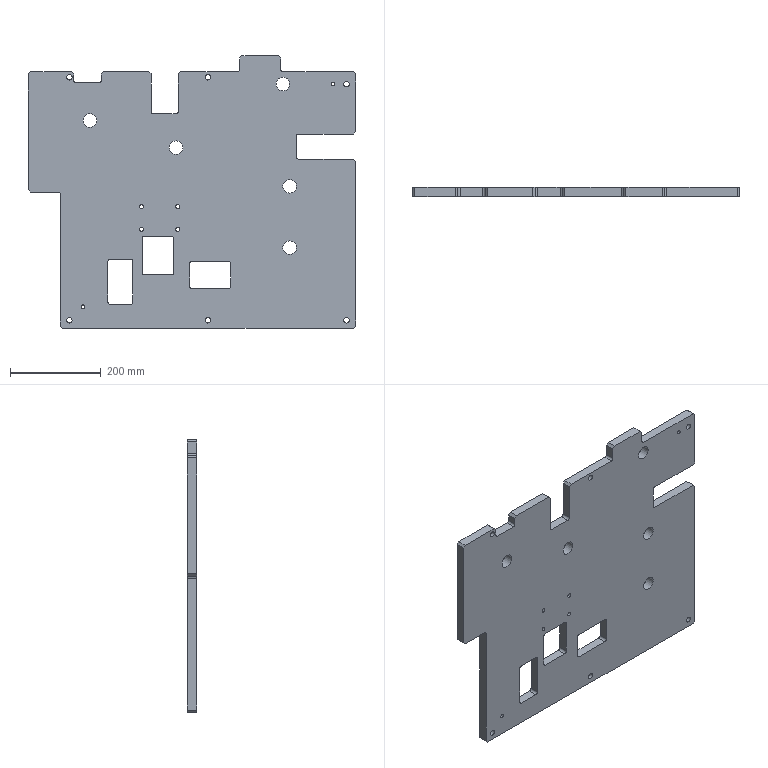Part | NX | features BREP 1 | 1 solid | 345 faces | box 720 x 20 x 600 mm | volume 7014374 mm3 | cylinder 167 | cone 123 | plane 55 | commonest cylinder face diameters 6 x72 5 x45 10 x21 4.2 x6 12 x6 18 x6